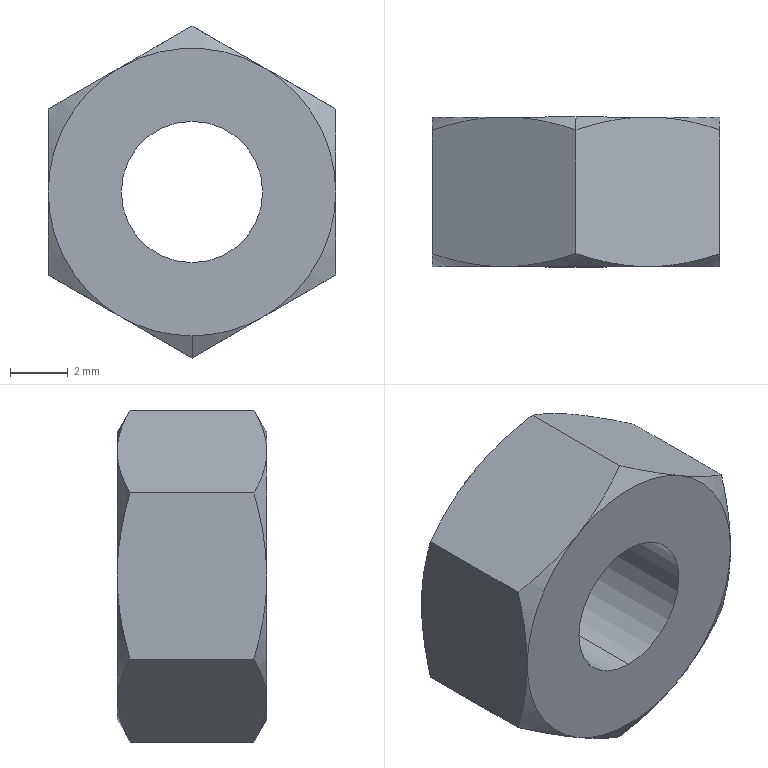Part | STEP file | 1 solid | 24 faces | box 10 x 5.2 x 11.547 mm | volume 349.391 mm3 | cone 14 | plane 8 | cylinder 2 | commonest cylinder face diameters 4.918 x2
STEP:
#1=CARTESIAN_POINT('',(2.5,0.,-4.33));
#2=VERTEX_POINT('',#1);
#3=CARTESIAN_POINT('',(0.,0.,-5.));
#4=VERTEX_POINT('',#3);
#5=CARTESIAN_POINT('',(0.,0.,0.));
#6=DIRECTION('',(0.,1.,0.));
#7=DIRECTION('',(0.,0.,1.));
#8=AXIS2_PLACEMENT_3D('',#5,#6,#7);
#9=CIRCLE('',#8,5.);
#10=EDGE_CURVE('',#2,#4,#9,.T.);
#11=ORIENTED_EDGE('',*,*,#10,.T.);
#12=CARTESIAN_POINT('',(0.,0.4466,-5.774));
#13=VERTEX_POINT('',#12);
#14=CARTESIAN_POINT('',(0.,0.,-5.));
#15=DIRECTION('',(0.,0.5,-0.866));
#16=VECTOR('',#15,1000.);
#17=LINE('',#14,#16);
#18=EDGE_CURVE('',#4,#13,#17,.T.);
#19=ORIENTED_EDGE('',*,*,#18,.T.);
#20=CARTESIAN_POINT('',(0.,0.4466,-5.774));
#21=CARTESIAN_POINT('',(0.8179,0.1739,-5.301));
#22=CARTESIAN_POINT('',(1.648,0.,-4.822));
#23=CARTESIAN_POINT('',(2.5,0.,-4.33));
#24=B_SPLINE_CURVE_WITH_KNOTS('',3,(#20,#21,#22,#23),.UNSPECIFIED.,.F.,.F.,(4,4),(0.000000238,0.002921),.UNSPECIFIED.);
#25=EDGE_CURVE('',#13,#2,#24,.T.);
#26=ORIENTED_EDGE('',*,*,#25,.T.);
#27=EDGE_LOOP('',(#11,#19,#26));
#28=FACE_OUTER_BOUND('',#27,.T.);
#29=CARTESIAN_POINT('',(0.,0.,0.));
#30=DIRECTION('',(0.,1.,0.));
#31=DIRECTION('',(0.,0.,-1.));
#32=AXIS2_PLACEMENT_3D('',#29,#30,#31);
#33=CONICAL_SURFACE('',#32,5.,1.047);
#34=ADVANCED_FACE('',(#28),#33,.T.);
#35=CARTESIAN_POINT('',(0.,5.2,5.));
#36=VERTEX_POINT('',#35);
#37=CARTESIAN_POINT('',(2.5,5.2,4.33));
#38=VERTEX_POINT('',#37);
#39=CARTESIAN_POINT('',(0.,5.2,0.));
#40=DIRECTION('',(0.,1.,0.));
#41=DIRECTION('',(0.,0.,1.));
#42=AXIS2_PLACEMENT_3D('',#39,#40,#41);
#43=CIRCLE('',#42,5.);
#44=EDGE_CURVE('',#36,#38,#43,.T.);
#45=ORIENTED_EDGE('',*,*,#44,.F.);
#46=CARTESIAN_POINT('',(0.,4.753,5.774));
#47=VERTEX_POINT('',#46);
#48=CARTESIAN_POINT('',(0.,5.2,5.));
#49=DIRECTION('',(0.,-0.5,0.866));
#50=VECTOR('',#49,1000.);
#51=LINE('',#48,#50);
#52=EDGE_CURVE('',#36,#47,#51,.T.);
#53=ORIENTED_EDGE('',*,*,#52,.T.);
#54=CARTESIAN_POINT('',(0.,4.753,5.774));
#55=CARTESIAN_POINT('',(0.8179,5.026,5.301));
#56=CARTESIAN_POINT('',(1.648,5.2,4.822));
#57=CARTESIAN_POINT('',(2.5,5.2,4.33));
#58=B_SPLINE_CURVE_WITH_KNOTS('',3,(#54,#55,#56,#57),.UNSPECIFIED.,.F.,.F.,(4,4),(0.000000238,0.002921),.UNSPECIFIED.);
#59=EDGE_CURVE('',#47,#38,#58,.T.);
#60=ORIENTED_EDGE('',*,*,#59,.T.);
#61=EDGE_LOOP('',(#45,#53,#60));
#62=FACE_OUTER_BOUND('',#61,.T.);
#63=CARTESIAN_POINT('',(0.,5.2,0.));
#64=DIRECTION('',(0.,-1.,0.));
#65=DIRECTION('',(0.,0.,1.));
#66=AXIS2_PLACEMENT_3D('',#63,#64,#65);
#67=CONICAL_SURFACE('',#66,5.,1.047);
#68=ADVANCED_FACE('',(#62),#67,.T.);
#69=CARTESIAN_POINT('',(0.,5.2,-2.459));
#70=VERTEX_POINT('',#69);
#71=CARTESIAN_POINT('',(0.,5.2,2.459));
#72=VERTEX_POINT('',#71);
#73=CARTESIAN_POINT('',(0.,5.2,0.));
#74=DIRECTION('',(0.,1.,0.));
#75=DIRECTION('',(0.,0.,1.));
#76=AXIS2_PLACEMENT_3D('',#73,#74,#75);
#77=CIRCLE('',#76,2.459);
#78=EDGE_CURVE('',#70,#72,#77,.T.);
#79=ORIENTED_EDGE('',*,*,#78,.T.);
#80=CARTESIAN_POINT('',(0.,0.,2.459));
#81=VERTEX_POINT('',#80);
#82=CARTESIAN_POINT('',(0.,5.2,2.459));
#83=DIRECTION('',(0.,-1.,0.));
#84=VECTOR('',#83,1000.);
#85=LINE('',#82,#84);
#86=EDGE_CURVE('',#72,#81,#85,.T.);
#87=ORIENTED_EDGE('',*,*,#86,.T.);
#88=CARTESIAN_POINT('',(0.,0.,-2.459));
#89=VERTEX_POINT('',#88);
#90=CARTESIAN_POINT('',(0.,0.,0.));
#91=DIRECTION('',(0.,1.,0.));
#92=DIRECTION('',(0.,0.,1.));
#93=AXIS2_PLACEMENT_3D('',#90,#91,#92);
#94=CIRCLE('',#93,2.459);
#95=EDGE_CURVE('',#89,#81,#94,.T.);
#96=ORIENTED_EDGE('',*,*,#95,.F.);
#97=CARTESIAN_POINT('',(0.,5.2,-2.459));
#98=DIRECTION('',(0.,-1.,0.));
#99=VECTOR('',#98,1000.);
#100=LINE('',#97,#99);
#101=EDGE_CURVE('',#70,#89,#100,.T.);
#102=ORIENTED_EDGE('',*,*,#101,.F.);
#103=EDGE_LOOP('',(#79,#87,#96,#102));
#104=FACE_OUTER_BOUND('',#103,.T.);
#105=CARTESIAN_POINT('',(0.,5.2,0.));
#106=DIRECTION('',(0.,-1.,0.));
#107=DIRECTION('',(0.,0.,-1.));
#108=AXIS2_PLACEMENT_3D('',#105,#106,#107);
#109=CYLINDRICAL_SURFACE('',#108,2.459);
#110=ADVANCED_FACE('',(#104),#109,.F.);
#111=CARTESIAN_POINT('',(-5.,0.4466,-2.887));
#112=VERTEX_POINT('',#111);
#113=CARTESIAN_POINT('',(-2.5,0.,-4.33));
#114=VERTEX_POINT('',#113);
#115=CARTESIAN_POINT('',(-5.,0.4466,-2.887));
#116=CARTESIAN_POINT('',(-4.182,0.1739,-3.359));
#117=CARTESIAN_POINT('',(-3.352,0.,-3.838));
#118=CARTESIAN_POINT('',(-2.5,0.,-4.33));
#119=B_SPLINE_CURVE_WITH_KNOTS('',3,(#115,#116,#117,#118),.UNSPECIFIED.,.F.,.F.,(4,4),(0.000000238,0.002921),.UNSPECIFIED.);
#120=EDGE_CURVE('',#112,#114,#119,.T.);
#121=ORIENTED_EDGE('',*,*,#120,.F.);
#122=CARTESIAN_POINT('',(-5.,4.753,-2.887));
#123=VERTEX_POINT('',#122);
#124=CARTESIAN_POINT('',(-5.,5.2,-2.887));
#125=DIRECTION('',(0.,-1.,0.));
#126=VECTOR('',#125,1000.);
#127=LINE('',#124,#126);
#128=EDGE_CURVE('',#123,#112,#127,.T.);
#129=ORIENTED_EDGE('',*,*,#128,.F.);
#130=CARTESIAN_POINT('',(-2.5,5.2,-4.33));
#131=VERTEX_POINT('',#130);
#132=CARTESIAN_POINT('',(-2.5,5.2,-4.33));
#133=CARTESIAN_POINT('',(-2.712,5.2,-4.208));
#134=CARTESIAN_POINT('',(-2.925,5.189,-4.085));
#135=CARTESIAN_POINT('',(-3.347,5.149,-3.841));
#136=CARTESIAN_POINT('',(-3.556,5.118,-3.72));
#137=CARTESIAN_POINT('',(-4.181,5.002,-3.36));
#138=CARTESIAN_POINT('',(-4.592,4.889,-3.122));
#139=CARTESIAN_POINT('',(-5.,4.753,-2.887));
#140=B_SPLINE_CURVE_WITH_KNOTS('',3,(#132,#133,#134,#135,#136,#137,#138,#139),.UNSPECIFIED.,.F.,.F.,(4,2,2,4),(0.002921,0.003649,0.004376,0.005831),.UNSPECIFIED.);
#141=EDGE_CURVE('',#131,#123,#140,.T.);
#142=ORIENTED_EDGE('',*,*,#141,.F.);
#143=CARTESIAN_POINT('',(0.,4.753,-5.774));
#144=VERTEX_POINT('',#143);
#145=CARTESIAN_POINT('',(0.,4.753,-5.774));
#146=CARTESIAN_POINT('',(-0.8179,5.026,-5.301));
#147=CARTESIAN_POINT('',(-1.648,5.2,-4.822));
#148=CARTESIAN_POINT('',(-2.5,5.2,-4.33));
#149=B_SPLINE_CURVE_WITH_KNOTS('',3,(#145,#146,#147,#148),.UNSPECIFIED.,.F.,.F.,(4,4),(0.000000238,0.002921),.UNSPECIFIED.);
#150=EDGE_CURVE('',#144,#131,#149,.T.);
#151=ORIENTED_EDGE('',*,*,#150,.F.);
#152=CARTESIAN_POINT('',(0.,5.2,-5.774));
#153=DIRECTION('',(0.,-1.,0.));
#154=VECTOR('',#153,1000.);
#155=LINE('',#152,#154);
#156=EDGE_CURVE('',#144,#13,#155,.T.);
#157=ORIENTED_EDGE('',*,*,#156,.T.);
#158=CARTESIAN_POINT('',(-2.5,0.,-4.33));
#159=CARTESIAN_POINT('',(-2.288,0.,-4.453));
#160=CARTESIAN_POINT('',(-2.075,0.01056,-4.576));
#161=CARTESIAN_POINT('',(-1.653,0.0514,-4.819));
#162=CARTESIAN_POINT('',(-1.444,0.08166,-4.94));
#163=CARTESIAN_POINT('',(-0.8193,0.1983,-5.3));
#164=CARTESIAN_POINT('',(-0.4079,0.3106,-5.538));
#165=CARTESIAN_POINT('',(0.,0.4466,-5.774));
#166=B_SPLINE_CURVE_WITH_KNOTS('',3,(#158,#159,#160,#161,#162,#163,#164,#165),.UNSPECIFIED.,.F.,.F.,(4,2,2,4),(0.002921,0.003649,0.004376,0.005831),.UNSPECIFIED.);
#167=EDGE_CURVE('',#114,#13,#166,.T.);
#168=ORIENTED_EDGE('',*,*,#167,.F.);
#169=EDGE_LOOP('',(#121,#129,#142,#151,#157,#168));
#170=FACE_OUTER_BOUND('',#169,.T.);
#171=CARTESIAN_POINT('',(0.,5.2,-5.774));
#172=DIRECTION('',(0.5,0.,0.866));
#173=DIRECTION('',(0.866,0.,-0.5));
#174=AXIS2_PLACEMENT_3D('',#171,#172,#173);
#175=PLANE('',#174);
#176=ADVANCED_FACE('',(#170),#175,.F.);
#177=CARTESIAN_POINT('',(-5.,0.4466,2.887));
#178=VERTEX_POINT('',#177);
#179=CARTESIAN_POINT('',(-5.,0.,0.));
#180=VERTEX_POINT('',#179);
#181=CARTESIAN_POINT('',(-5.,0.4466,2.887));
#182=CARTESIAN_POINT('',(-5.,0.3118,2.42));
#183=CARTESIAN_POINT('',(-5.,0.1996,1.947));
#184=CARTESIAN_POINT('',(-5.,0.04317,0.9834));
#185=CARTESIAN_POINT('',(-5.,0.,0.4885));
#186=CARTESIAN_POINT('',(-5.,0.,0.));
#187=B_SPLINE_CURVE_WITH_KNOTS('',3,(#181,#182,#183,#184,#185,#186),.UNSPECIFIED.,.F.,.F.,(4,2,4),(0.01606,0.01752,0.01898),.UNSPECIFIED.);
#188=EDGE_CURVE('',#178,#180,#187,.T.);
#189=ORIENTED_EDGE('',*,*,#188,.F.);
#190=CARTESIAN_POINT('',(-5.,4.753,2.887));
#191=VERTEX_POINT('',#190);
#192=CARTESIAN_POINT('',(-5.,5.2,2.887));
#193=DIRECTION('',(0.,-1.,0.));
#194=VECTOR('',#193,1000.);
#195=LINE('',#192,#194);
#196=EDGE_CURVE('',#191,#178,#195,.T.);
#197=ORIENTED_EDGE('',*,*,#196,.F.);
#198=CARTESIAN_POINT('',(-5.,5.2,0.));
#199=VERTEX_POINT('',#198);
#200=CARTESIAN_POINT('',(-5.,5.2,0.));
#201=CARTESIAN_POINT('',(-5.,5.2,0.4885));
#202=CARTESIAN_POINT('',(-5.,5.157,0.9834));
#203=CARTESIAN_POINT('',(-5.,5.,1.947));
#204=CARTESIAN_POINT('',(-5.,4.888,2.42));
#205=CARTESIAN_POINT('',(-5.,4.753,2.887));
#206=B_SPLINE_CURVE_WITH_KNOTS('',3,(#200,#201,#202,#203,#204,#205),.UNSPECIFIED.,.F.,.F.,(4,2,4),(0.008187,0.009649,0.01111),.UNSPECIFIED.);
#207=EDGE_CURVE('',#199,#191,#206,.T.);
#208=ORIENTED_EDGE('',*,*,#207,.F.);
#209=CARTESIAN_POINT('',(-5.,4.753,-2.887));
#210=CARTESIAN_POINT('',(-5.,4.889,-2.417));
#211=CARTESIAN_POINT('',(-5.,5.003,-1.936));
#212=CARTESIAN_POINT('',(-5.,5.158,-0.9728));
#213=CARTESIAN_POINT('',(-5.,5.2,-0.4881));
#214=CARTESIAN_POINT('',(-5.,5.2,0.));
#215=B_SPLINE_CURVE_WITH_KNOTS('',3,(#209,#210,#211,#212,#213,#214),.UNSPECIFIED.,.F.,.F.,(4,2,4),(0.005265,0.006726,0.008187),.UNSPECIFIED.);
#216=EDGE_CURVE('',#123,#199,#215,.T.);
#217=ORIENTED_EDGE('',*,*,#216,.F.);
#218=ORIENTED_EDGE('',*,*,#128,.T.);
#219=CARTESIAN_POINT('',(-5.,0.,0.));
#220=CARTESIAN_POINT('',(-5.,0.,-0.4881));
#221=CARTESIAN_POINT('',(-5.,0.04198,-0.9728));
#222=CARTESIAN_POINT('',(-5.,0.1973,-1.936));
#223=CARTESIAN_POINT('',(-5.,0.311,-2.417));
#224=CARTESIAN_POINT('',(-5.,0.4466,-2.887));
#225=B_SPLINE_CURVE_WITH_KNOTS('',3,(#219,#220,#221,#222,#223,#224),.UNSPECIFIED.,.F.,.F.,(4,2,4),(0.01898,0.02045,0.02191),.UNSPECIFIED.);
#226=EDGE_CURVE('',#180,#112,#225,.T.);
#227=ORIENTED_EDGE('',*,*,#226,.F.);
#228=EDGE_LOOP('',(#189,#197,#208,#217,#218,#227));
#229=FACE_OUTER_BOUND('',#228,.T.);
#230=CARTESIAN_POINT('',(-5.,5.2,-2.887));
#231=DIRECTION('',(1.,0.,0.));
#232=DIRECTION('',(0.,0.,-1.));
#233=AXIS2_PLACEMENT_3D('',#230,#231,#232);
#234=PLANE('',#233);
#235=ADVANCED_FACE('',(#229),#234,.F.);
#236=CARTESIAN_POINT('',(0.,0.4466,5.774));
#237=VERTEX_POINT('',#236);
#238=CARTESIAN_POINT('',(-2.5,0.,4.33));
#239=VERTEX_POINT('',#238);
#240=CARTESIAN_POINT('',(0.,0.4466,5.774));
#241=CARTESIAN_POINT('',(-0.8179,0.1739,5.301));
#242=CARTESIAN_POINT('',(-1.648,0.,4.822));
#243=CARTESIAN_POINT('',(-2.5,0.,4.33));
#244=B_SPLINE_CURVE_WITH_KNOTS('',3,(#240,#241,#242,#243),.UNSPECIFIED.,.F.,.F.,(4,4),(0.000000238,0.002921),.UNSPECIFIED.);
#245=EDGE_CURVE('',#237,#239,#244,.T.);
#246=ORIENTED_EDGE('',*,*,#245,.F.);
#247=CARTESIAN_POINT('',(0.,5.2,5.774));
#248=DIRECTION('',(0.,-1.,0.));
#249=VECTOR('',#248,1000.);
#250=LINE('',#247,#249);
#251=EDGE_CURVE('',#47,#237,#250,.T.);
#252=ORIENTED_EDGE('',*,*,#251,.F.);
#253=CARTESIAN_POINT('',(-2.5,5.2,4.33));
#254=VERTEX_POINT('',#253);
#255=CARTESIAN_POINT('',(-2.5,5.2,4.33));
#256=CARTESIAN_POINT('',(-2.288,5.2,4.453));
#257=CARTESIAN_POINT('',(-2.075,5.189,4.576));
#258=CARTESIAN_POINT('',(-1.653,5.149,4.819));
#259=CARTESIAN_POINT('',(-1.444,5.118,4.94));
#260=CARTESIAN_POINT('',(-0.8193,5.002,5.3));
#261=CARTESIAN_POINT('',(-0.4079,4.889,5.538));
#262=CARTESIAN_POINT('',(0.,4.753,5.774));
#263=B_SPLINE_CURVE_WITH_KNOTS('',3,(#255,#256,#257,#258,#259,#260,#261,#262),.UNSPECIFIED.,.F.,.F.,(4,2,2,4),(0.002921,0.003649,0.004376,0.005831),.UNSPECIFIED.);
#264=EDGE_CURVE('',#254,#47,#263,.T.);
#265=ORIENTED_EDGE('',*,*,#264,.F.);
#266=CARTESIAN_POINT('',(-5.,4.753,2.887));
#267=CARTESIAN_POINT('',(-4.182,5.026,3.359));
#268=CARTESIAN_POINT('',(-3.352,5.2,3.838));
#269=CARTESIAN_POINT('',(-2.5,5.2,4.33));
#270=B_SPLINE_CURVE_WITH_KNOTS('',3,(#266,#267,#268,#269),.UNSPECIFIED.,.F.,.F.,(4,4),(0.000000238,0.002921),.UNSPECIFIED.);
#271=EDGE_CURVE('',#191,#254,#270,.T.);
#272=ORIENTED_EDGE('',*,*,#271,.F.);
#273=ORIENTED_EDGE('',*,*,#196,.T.);
#274=CARTESIAN_POINT('',(-2.5,0.,4.33));
#275=CARTESIAN_POINT('',(-2.712,0.,4.208));
#276=CARTESIAN_POINT('',(-2.925,0.01056,4.085));
#277=CARTESIAN_POINT('',(-3.347,0.0514,3.841));
#278=CARTESIAN_POINT('',(-3.556,0.08166,3.72));
#279=CARTESIAN_POINT('',(-4.181,0.1983,3.36));
#280=CARTESIAN_POINT('',(-4.592,0.3106,3.122));
#281=CARTESIAN_POINT('',(-5.,0.4466,2.887));
#282=B_SPLINE_CURVE_WITH_KNOTS('',3,(#274,#275,#276,#277,#278,#279,#280,#281),.UNSPECIFIED.,.F.,.F.,(4,2,2,4),(0.002921,0.003649,0.004376,0.005831),.UNSPECIFIED.);
#283=EDGE_CURVE('',#239,#178,#282,.T.);
#284=ORIENTED_EDGE('',*,*,#283,.F.);
#285=EDGE_LOOP('',(#246,#252,#265,#272,#273,#284));
#286=FACE_OUTER_BOUND('',#285,.T.);
#287=CARTESIAN_POINT('',(-5.,5.2,2.887));
#288=DIRECTION('',(0.5,0.,-0.866));
#289=DIRECTION('',(-0.866,0.,-0.5));
#290=AXIS2_PLACEMENT_3D('',#287,#288,#289);
#291=PLANE('',#290);
#292=ADVANCED_FACE('',(#286),#291,.F.);
#293=CARTESIAN_POINT('',(5.,0.4466,2.887));
#294=VERTEX_POINT('',#293);
#295=CARTESIAN_POINT('',(2.5,0.,4.33));
#296=VERTEX_POINT('',#295);
#297=CARTESIAN_POINT('',(5.,0.4466,2.887));
#298=CARTESIAN_POINT('',(4.182,0.1739,3.359));
#299=CARTESIAN_POINT('',(3.352,0.,3.838));
#300=CARTESIAN_POINT('',(2.5,0.,4.33));
#301=B_SPLINE_CURVE_WITH_KNOTS('',3,(#297,#298,#299,#300),.UNSPECIFIED.,.F.,.F.,(4,4),(0.000000238,0.002921),.UNSPECIFIED.);
#302=EDGE_CURVE('',#294,#296,#301,.T.);
#303=ORIENTED_EDGE('',*,*,#302,.F.);
#304=CARTESIAN_POINT('',(5.,4.753,2.887));
#305=VERTEX_POINT('',#304);
#306=CARTESIAN_POINT('',(5.,5.2,2.887));
#307=DIRECTION('',(0.,-1.,0.));
#308=VECTOR('',#307,1000.);
#309=LINE('',#306,#308);
#310=EDGE_CURVE('',#305,#294,#309,.T.);
#311=ORIENTED_EDGE('',*,*,#310,.F.);
#312=CARTESIAN_POINT('',(2.5,5.2,4.33));
#313=CARTESIAN_POINT('',(2.712,5.2,4.208));
#314=CARTESIAN_POINT('',(2.925,5.189,4.085));
#315=CARTESIAN_POINT('',(3.347,5.149,3.841));
#316=CARTESIAN_POINT('',(3.556,5.118,3.72));
#317=CARTESIAN_POINT('',(4.181,5.002,3.36));
#318=CARTESIAN_POINT('',(4.592,4.889,3.122));
#319=CARTESIAN_POINT('',(5.,4.753,2.887));
#320=B_SPLINE_CURVE_WITH_KNOTS('',3,(#312,#313,#314,#315,#316,#317,#318,#319),.UNSPECIFIED.,.F.,.F.,(4,2,2,4),(0.002921,0.003649,0.004376,0.005831),.UNSPECIFIED.);
#321=EDGE_CURVE('',#38,#305,#320,.T.);
#322=ORIENTED_EDGE('',*,*,#321,.F.);
#323=ORIENTED_EDGE('',*,*,#59,.F.);
#324=ORIENTED_EDGE('',*,*,#251,.T.);
#325=CARTESIAN_POINT('',(2.5,0.,4.33));
#326=CARTESIAN_POINT('',(2.288,0.,4.453));
#327=CARTESIAN_POINT('',(2.075,0.01056,4.576));
#328=CARTESIAN_POINT('',(1.653,0.0514,4.819));
#329=CARTESIAN_POINT('',(1.444,0.08166,4.94));
#330=CARTESIAN_POINT('',(0.8193,0.1983,5.3));
#331=CARTESIAN_POINT('',(0.4079,0.3106,5.538));
#332=CARTESIAN_POINT('',(0.,0.4466,5.774));
#333=B_SPLINE_CURVE_WITH_KNOTS('',3,(#325,#326,#327,#328,#329,#330,#331,#332),.UNSPECIFIED.,.F.,.F.,(4,2,2,4),(0.002921,0.003649,0.004376,0.005831),.UNSPECIFIED.);
#334=EDGE_CURVE('',#296,#237,#333,.T.);
#335=ORIENTED_EDGE('',*,*,#334,.F.);
#336=EDGE_LOOP('',(#303,#311,#322,#323,#324,#335));
#337=FACE_OUTER_BOUND('',#336,.T.);
#338=CARTESIAN_POINT('',(0.,5.2,5.774));
#339=DIRECTION('',(-0.5,0.,-0.866));
#340=DIRECTION('',(-0.866,0.,0.5));
#341=AXIS2_PLACEMENT_3D('',#338,#339,#340);
#342=PLANE('',#341);
#343=ADVANCED_FACE('',(#337),#342,.F.);
#344=CARTESIAN_POINT('',(5.,0.4466,-2.887));
#345=VERTEX_POINT('',#344);
#346=CARTESIAN_POINT('',(5.,0.,0.));
#347=VERTEX_POINT('',#346);
#348=CARTESIAN_POINT('',(5.,0.4466,-2.887));
#349=CARTESIAN_POINT('',(5.,0.311,-2.417));
#350=CARTESIAN_POINT('',(5.,0.1973,-1.936));
#351=CARTESIAN_POINT('',(5.,0.04198,-0.9728));
#352=CARTESIAN_POINT('',(5.,0.,-0.4881));
#353=CARTESIAN_POINT('',(5.,0.,0.));
#354=B_SPLINE_CURVE_WITH_KNOTS('',3,(#348,#349,#350,#351,#352,#353),.UNSPECIFIED.,.F.,.F.,(4,2,4),(0.005265,0.006726,0.008187),.UNSPECIFIED.);
#355=EDGE_CURVE('',#345,#347,#354,.T.);
#356=ORIENTED_EDGE('',*,*,#355,.F.);
#357=CARTESIAN_POINT('',(5.,4.753,-2.887));
#358=VERTEX_POINT('',#357);
#359=CARTESIAN_POINT('',(5.,5.2,-2.887));
#360=DIRECTION('',(0.,-1.,0.));
#361=VECTOR('',#360,1000.);
#362=LINE('',#359,#361);
#363=EDGE_CURVE('',#358,#345,#362,.T.);
#364=ORIENTED_EDGE('',*,*,#363,.F.);
#365=CARTESIAN_POINT('',(5.,5.2,0.));
#366=VERTEX_POINT('',#365);
#367=CARTESIAN_POINT('',(5.,5.2,0.));
#368=CARTESIAN_POINT('',(5.,5.2,-0.4881));
#369=CARTESIAN_POINT('',(5.,5.158,-0.9728));
#370=CARTESIAN_POINT('',(5.,5.003,-1.936));
#371=CARTESIAN_POINT('',(5.,4.889,-2.417));
#372=CARTESIAN_POINT('',(5.,4.753,-2.887));
#373=B_SPLINE_CURVE_WITH_KNOTS('',3,(#367,#368,#369,#370,#371,#372),.UNSPECIFIED.,.F.,.F.,(4,2,4),(0.01898,0.02045,0.02191),.UNSPECIFIED.);
#374=EDGE_CURVE('',#366,#358,#373,.T.);
#375=ORIENTED_EDGE('',*,*,#374,.F.);
#376=CARTESIAN_POINT('',(5.,4.753,2.887));
#377=CARTESIAN_POINT('',(5.,4.888,2.42));
#378=CARTESIAN_POINT('',(5.,5.,1.947));
#379=CARTESIAN_POINT('',(5.,5.157,0.9834));
#380=CARTESIAN_POINT('',(5.,5.2,0.4885));
#381=CARTESIAN_POINT('',(5.,5.2,0.));
#382=B_SPLINE_CURVE_WITH_KNOTS('',3,(#376,#377,#378,#379,#380,#381),.UNSPECIFIED.,.F.,.F.,(4,2,4),(0.01606,0.01752,0.01898),.UNSPECIFIED.);
#383=EDGE_CURVE('',#305,#366,#382,.T.);
#384=ORIENTED_EDGE('',*,*,#383,.F.);
#385=ORIENTED_EDGE('',*,*,#310,.T.);
#386=CARTESIAN_POINT('',(5.,0.,0.));
#387=CARTESIAN_POINT('',(5.,0.,0.4885));
#388=CARTESIAN_POINT('',(5.,0.04317,0.9834));
#389=CARTESIAN_POINT('',(5.,0.1996,1.947));
#390=CARTESIAN_POINT('',(5.,0.3118,2.42));
#391=CARTESIAN_POINT('',(5.,0.4466,2.887));
#392=B_SPLINE_CURVE_WITH_KNOTS('',3,(#386,#387,#388,#389,#390,#391),.UNSPECIFIED.,.F.,.F.,(4,2,4),(0.008187,0.009649,0.01111),.UNSPECIFIED.);
#393=EDGE_CURVE('',#347,#294,#392,.T.);
#394=ORIENTED_EDGE('',*,*,#393,.F.);
#395=EDGE_LOOP('',(#356,#364,#375,#384,#385,#394));
#396=FACE_OUTER_BOUND('',#395,.T.);
#397=CARTESIAN_POINT('',(5.,5.2,2.887));
#398=DIRECTION('',(-1.,0.,0.));
#399=DIRECTION('',(0.,0.,1.));
#400=AXIS2_PLACEMENT_3D('',#397,#398,#399);
#401=PLANE('',#400);
#402=ADVANCED_FACE('',(#396),#401,.F.);
#403=ORIENTED_EDGE('',*,*,#25,.F.);
#404=ORIENTED_EDGE('',*,*,#156,.F.);
#405=CARTESIAN_POINT('',(2.5,5.2,-4.33));
#406=VERTEX_POINT('',#405);
#407=CARTESIAN_POINT('',(2.5,5.2,-4.33));
#408=CARTESIAN_POINT('',(2.288,5.2,-4.453));
#409=CARTESIAN_POINT('',(2.075,5.189,-4.576));
#410=CARTESIAN_POINT('',(1.653,5.149,-4.819));
#411=CARTESIAN_POINT('',(1.444,5.118,-4.94));
#412=CARTESIAN_POINT('',(0.8193,5.002,-5.3));
#413=CARTESIAN_POINT('',(0.4079,4.889,-5.538));
#414=CARTESIAN_POINT('',(0.,4.753,-5.774));
#415=B_SPLINE_CURVE_WITH_KNOTS('',3,(#407,#408,#409,#410,#411,#412,#413,#414),.UNSPECIFIED.,.F.,.F.,(4,2,2,4),(0.002921,0.003649,0.004376,0.005831),.UNSPECIFIED.);
#416=EDGE_CURVE('',#406,#144,#415,.T.);
#417=ORIENTED_EDGE('',*,*,#416,.F.);
#418=CARTESIAN_POINT('',(5.,4.753,-2.887));
#419=CARTESIAN_POINT('',(4.182,5.026,-3.359));
#420=CARTESIAN_POINT('',(3.352,5.2,-3.838));
#421=CARTESIAN_POINT('',(2.5,5.2,-4.33));
#422=B_SPLINE_CURVE_WITH_KNOTS('',3,(#418,#419,#420,#421),.UNSPECIFIED.,.F.,.F.,(4,4),(0.000000238,0.002921),.UNSPECIFIED.);
#423=EDGE_CURVE('',#358,#406,#422,.T.);
#424=ORIENTED_EDGE('',*,*,#423,.F.);
#425=ORIENTED_EDGE('',*,*,#363,.T.);
#426=CARTESIAN_POINT('',(2.5,0.,-4.33));
#427=CARTESIAN_POINT('',(2.712,0.,-4.208));
#428=CARTESIAN_POINT('',(2.925,0.01056,-4.085));
#429=CARTESIAN_POINT('',(3.347,0.0514,-3.841));
#430=CARTESIAN_POINT('',(3.556,0.08166,-3.72));
#431=CARTESIAN_POINT('',(4.181,0.1983,-3.36));
#432=CARTESIAN_POINT('',(4.592,0.3106,-3.122));
#433=CARTESIAN_POINT('',(5.,0.4466,-2.887));
#434=B_SPLINE_CURVE_WITH_KNOTS('',3,(#426,#427,#428,#429,#430,#431,#432,#433),.UNSPECIFIED.,.F.,.F.,(4,2,2,4),(0.002921,0.003649,0.004376,0.005831),.UNSPECIFIED.);
#435=EDGE_CURVE('',#2,#345,#434,.T.);
#436=ORIENTED_EDGE('',*,*,#435,.F.);
#437=EDGE_LOOP('',(#403,#404,#417,#424,#425,#436));
#438=FACE_OUTER_BOUND('',#437,.T.);
#439=CARTESIAN_POINT('',(5.,5.2,-2.887));
#440=DIRECTION('',(-0.5,0.,0.866));
#441=DIRECTION('',(0.866,0.,0.5));
#442=AXIS2_PLACEMENT_3D('',#439,#440,#441);
#443=PLANE('',#442);
#444=ADVANCED_FACE('',(#438),#443,.F.);
#445=ORIENTED_EDGE('',*,*,#95,.T.);
#446=CARTESIAN_POINT('',(0.,0.,0.));
#447=DIRECTION('',(0.,1.,0.));
#448=DIRECTION('',(0.,0.,1.));
#449=AXIS2_PLACEMENT_3D('',#446,#447,#448);
#450=CIRCLE('',#449,2.459);
#451=EDGE_CURVE('',#81,#89,#450,.T.);
#452=ORIENTED_EDGE('',*,*,#451,.T.);
#453=EDGE_LOOP('',(#445,#452));
#454=FACE_BOUND('',#453,.T.);
#455=CARTESIAN_POINT('',(0.,0.,0.));
#456=DIRECTION('',(0.,1.,0.));
#457=DIRECTION('',(0.,0.,1.));
#458=AXIS2_PLACEMENT_3D('',#455,#456,#457);
#459=CIRCLE('',#458,5.);
#460=EDGE_CURVE('',#296,#347,#459,.T.);
#461=ORIENTED_EDGE('',*,*,#460,.F.);
#462=CARTESIAN_POINT('',(0.,0.,0.));
#463=DIRECTION('',(0.,1.,0.));
#464=DIRECTION('',(0.,0.,1.));
#465=AXIS2_PLACEMENT_3D('',#462,#463,#464);
#466=CIRCLE('',#465,5.);
#467=EDGE_CURVE('',#239,#296,#466,.T.);
#468=ORIENTED_EDGE('',*,*,#467,.F.);
#469=CARTESIAN_POINT('',(0.,0.,0.));
#470=DIRECTION('',(0.,1.,0.));
#471=DIRECTION('',(0.,0.,1.));
#472=AXIS2_PLACEMENT_3D('',#469,#470,#471);
#473=CIRCLE('',#472,5.);
#474=EDGE_CURVE('',#180,#239,#473,.T.);
#475=ORIENTED_EDGE('',*,*,#474,.F.);
#476=CARTESIAN_POINT('',(0.,0.,0.));
#477=DIRECTION('',(0.,1.,0.));
#478=DIRECTION('',(0.,0.,1.));
#479=AXIS2_PLACEMENT_3D('',#476,#477,#478);
#480=CIRCLE('',#479,5.);
#481=EDGE_CURVE('',#114,#180,#480,.T.);
#482=ORIENTED_EDGE('',*,*,#481,.F.);
#483=CARTESIAN_POINT('',(0.,0.,0.));
#484=DIRECTION('',(0.,1.,0.));
#485=DIRECTION('',(0.,0.,1.));
#486=AXIS2_PLACEMENT_3D('',#483,#484,#485);
#487=CIRCLE('',#486,5.);
#488=EDGE_CURVE('',#4,#114,#487,.T.);
#489=ORIENTED_EDGE('',*,*,#488,.F.);
#490=ORIENTED_EDGE('',*,*,#10,.F.);
#491=CARTESIAN_POINT('',(0.,0.,0.));
#492=DIRECTION('',(0.,-1.,0.));
#493=DIRECTION('',(0.,0.,-1.));
#494=AXIS2_PLACEMENT_3D('',#491,#492,#493);
#495=CIRCLE('',#494,5.);
#496=EDGE_CURVE('',#2,#347,#495,.T.);
#497=ORIENTED_EDGE('',*,*,#496,.T.);
#498=EDGE_LOOP('',(#461,#468,#475,#482,#489,#490,#497));
#499=FACE_OUTER_BOUND('',#498,.T.);
#500=CARTESIAN_POINT('',(0.,0.,0.));
#501=DIRECTION('',(0.,1.,0.));
#502=DIRECTION('',(0.,0.,1.));
#503=AXIS2_PLACEMENT_3D('',#500,#501,#502);
#504=PLANE('',#503);
#505=ADVANCED_FACE('',(#454,#499),#504,.F.);
#506=ORIENTED_EDGE('',*,*,#78,.F.);
#507=CARTESIAN_POINT('',(0.,5.2,0.));
#508=DIRECTION('',(0.,1.,0.));
#509=DIRECTION('',(0.,0.,1.));
#510=AXIS2_PLACEMENT_3D('',#507,#508,#509);
#511=CIRCLE('',#510,2.459);
#512=EDGE_CURVE('',#72,#70,#511,.T.);
#513=ORIENTED_EDGE('',*,*,#512,.F.);
#514=EDGE_LOOP('',(#506,#513));
#515=FACE_BOUND('',#514,.T.);
#516=CARTESIAN_POINT('',(0.,5.2,0.));
#517=DIRECTION('',(0.,1.,0.));
#518=DIRECTION('',(0.,0.,1.));
#519=AXIS2_PLACEMENT_3D('',#516,#517,#518);
#520=CIRCLE('',#519,5.);
#521=EDGE_CURVE('',#254,#36,#520,.T.);
#522=ORIENTED_EDGE('',*,*,#521,.T.);
#523=ORIENTED_EDGE('',*,*,#44,.T.);
#524=CARTESIAN_POINT('',(0.,5.2,0.));
#525=DIRECTION('',(0.,1.,0.));
#526=DIRECTION('',(0.,0.,1.));
#527=AXIS2_PLACEMENT_3D('',#524,#525,#526);
#528=CIRCLE('',#527,5.);
#529=EDGE_CURVE('',#38,#366,#528,.T.);
#530=ORIENTED_EDGE('',*,*,#529,.T.);
#531=CARTESIAN_POINT('',(0.,5.2,0.));
#532=DIRECTION('',(0.,1.,0.));
#533=DIRECTION('',(0.,0.,1.));
#534=AXIS2_PLACEMENT_3D('',#531,#532,#533);
#535=CIRCLE('',#534,5.);
#536=EDGE_CURVE('',#366,#406,#535,.T.);
#537=ORIENTED_EDGE('',*,*,#536,.T.);
#538=CARTESIAN_POINT('',(0.,5.2,0.));
#539=DIRECTION('',(0.,1.,0.));
#540=DIRECTION('',(0.,0.,1.));
#541=AXIS2_PLACEMENT_3D('',#538,#539,#540);
#542=CIRCLE('',#541,5.);
#543=EDGE_CURVE('',#406,#131,#542,.T.);
#544=ORIENTED_EDGE('',*,*,#543,.T.);
#545=CARTESIAN_POINT('',(0.,5.2,0.));
#546=DIRECTION('',(0.,1.,0.));
#547=DIRECTION('',(0.,0.,1.));
#548=AXIS2_PLACEMENT_3D('',#545,#546,#547);
#549=CIRCLE('',#548,5.);
#550=EDGE_CURVE('',#131,#199,#549,.T.);
#551=ORIENTED_EDGE('',*,*,#550,.T.);
#552=CARTESIAN_POINT('',(0.,5.2,0.));
#553=DIRECTION('',(0.,1.,0.));
#554=DIRECTION('',(0.,0.,1.));
#555=AXIS2_PLACEMENT_3D('',#552,#553,#554);
#556=CIRCLE('',#555,5.);
#557=EDGE_CURVE('',#199,#254,#556,.T.);
#558=ORIENTED_EDGE('',*,*,#557,.T.);
#559=EDGE_LOOP('',(#522,#523,#530,#537,#544,#551,#558));
#560=FACE_OUTER_BOUND('',#559,.T.);
#561=CARTESIAN_POINT('',(0.,5.2,0.));
#562=DIRECTION('',(0.,1.,0.));
#563=DIRECTION('',(0.,0.,1.));
#564=AXIS2_PLACEMENT_3D('',#561,#562,#563);
#565=PLANE('',#564);
#566=ADVANCED_FACE('',(#515,#560),#565,.T.);
#567=ORIENTED_EDGE('',*,*,#86,.F.);
#568=ORIENTED_EDGE('',*,*,#512,.T.);
#569=ORIENTED_EDGE('',*,*,#101,.T.);
#570=ORIENTED_EDGE('',*,*,#451,.F.);
#571=EDGE_LOOP('',(#567,#568,#569,#570));
#572=FACE_OUTER_BOUND('',#571,.T.);
#573=CARTESIAN_POINT('',(0.,5.2,0.));
#574=DIRECTION('',(0.,-1.,0.));
#575=DIRECTION('',(0.,0.,-1.));
#576=AXIS2_PLACEMENT_3D('',#573,#574,#575);
#577=CYLINDRICAL_SURFACE('',#576,2.459);
#578=ADVANCED_FACE('',(#572),#577,.F.);
#579=ORIENTED_EDGE('',*,*,#150,.T.);
#580=ORIENTED_EDGE('',*,*,#543,.F.);
#581=ORIENTED_EDGE('',*,*,#416,.T.);
#582=EDGE_LOOP('',(#579,#580,#581));
#583=FACE_OUTER_BOUND('',#582,.T.);
#584=CARTESIAN_POINT('',(0.,5.2,0.));
#585=DIRECTION('',(0.,-1.,0.));
#586=DIRECTION('',(0.,0.,1.));
#587=AXIS2_PLACEMENT_3D('',#584,#585,#586);
#588=CONICAL_SURFACE('',#587,5.,1.047);
#589=ADVANCED_FACE('',(#583),#588,.T.);
#590=ORIENTED_EDGE('',*,*,#374,.T.);
#591=ORIENTED_EDGE('',*,*,#423,.T.);
#592=ORIENTED_EDGE('',*,*,#536,.F.);
#593=EDGE_LOOP('',(#590,#591,#592));
#594=FACE_OUTER_BOUND('',#593,.T.);
#595=CARTESIAN_POINT('',(0.,5.2,0.));
#596=DIRECTION('',(0.,-1.,0.));
#597=DIRECTION('',(0.,0.,1.));
#598=AXIS2_PLACEMENT_3D('',#595,#596,#597);
#599=CONICAL_SURFACE('',#598,5.,1.047);
#600=ADVANCED_FACE('',(#594),#599,.T.);
#601=ORIENTED_EDGE('',*,*,#321,.T.);
#602=ORIENTED_EDGE('',*,*,#383,.T.);
#603=ORIENTED_EDGE('',*,*,#529,.F.);
#604=EDGE_LOOP('',(#601,#602,#603));
#605=FACE_OUTER_BOUND('',#604,.T.);
#606=CARTESIAN_POINT('',(0.,5.2,0.));
#607=DIRECTION('',(0.,-1.,0.));
#608=DIRECTION('',(0.,0.,1.));
#609=AXIS2_PLACEMENT_3D('',#606,#607,#608);
#610=CONICAL_SURFACE('',#609,5.,1.047);
#611=ADVANCED_FACE('',(#605),#610,.T.);
#612=ORIENTED_EDGE('',*,*,#52,.F.);
#613=ORIENTED_EDGE('',*,*,#521,.F.);
#614=ORIENTED_EDGE('',*,*,#264,.T.);
#615=EDGE_LOOP('',(#612,#613,#614));
#616=FACE_OUTER_BOUND('',#615,.T.);
#617=CARTESIAN_POINT('',(0.,5.2,0.));
#618=DIRECTION('',(0.,-1.,0.));
#619=DIRECTION('',(0.,0.,1.));
#620=AXIS2_PLACEMENT_3D('',#617,#618,#619);
#621=CONICAL_SURFACE('',#620,5.,1.047);
#622=ADVANCED_FACE('',(#616),#621,.T.);
#623=ORIENTED_EDGE('',*,*,#207,.T.);
#624=ORIENTED_EDGE('',*,*,#271,.T.);
#625=ORIENTED_EDGE('',*,*,#557,.F.);
#626=EDGE_LOOP('',(#623,#624,#625));
#627=FACE_OUTER_BOUND('',#626,.T.);
#628=CARTESIAN_POINT('',(0.,5.2,0.));
#629=DIRECTION('',(0.,-1.,0.));
#630=DIRECTION('',(0.,0.,1.));
#631=AXIS2_PLACEMENT_3D('',#628,#629,#630);
#632=CONICAL_SURFACE('',#631,5.,1.047);
#633=ADVANCED_FACE('',(#627),#632,.T.);
#634=ORIENTED_EDGE('',*,*,#141,.T.);
#635=ORIENTED_EDGE('',*,*,#216,.T.);
#636=ORIENTED_EDGE('',*,*,#550,.F.);
#637=EDGE_LOOP('',(#634,#635,#636));
#638=FACE_OUTER_BOUND('',#637,.T.);
#639=CARTESIAN_POINT('',(0.,5.2,0.));
#640=DIRECTION('',(0.,-1.,0.));
#641=DIRECTION('',(0.,0.,1.));
#642=AXIS2_PLACEMENT_3D('',#639,#640,#641);
#643=CONICAL_SURFACE('',#642,5.,1.047);
#644=ADVANCED_FACE('',(#638),#643,.T.);
#645=ORIENTED_EDGE('',*,*,#245,.T.);
#646=ORIENTED_EDGE('',*,*,#467,.T.);
#647=ORIENTED_EDGE('',*,*,#334,.T.);
#648=EDGE_LOOP('',(#645,#646,#647));
#649=FACE_OUTER_BOUND('',#648,.T.);
#650=CARTESIAN_POINT('',(0.,0.,0.));
#651=DIRECTION('',(0.,1.,0.));
#652=DIRECTION('',(0.,0.,-1.));
#653=AXIS2_PLACEMENT_3D('',#650,#651,#652);
#654=CONICAL_SURFACE('',#653,5.,1.047);
#655=ADVANCED_FACE('',(#649),#654,.T.);
#656=ORIENTED_EDGE('',*,*,#283,.T.);
#657=ORIENTED_EDGE('',*,*,#188,.T.);
#658=ORIENTED_EDGE('',*,*,#474,.T.);
#659=EDGE_LOOP('',(#656,#657,#658));
#660=FACE_OUTER_BOUND('',#659,.T.);
#661=CARTESIAN_POINT('',(0.,0.,0.));
#662=DIRECTION('',(0.,1.,0.));
#663=DIRECTION('',(0.,0.,-1.));
#664=AXIS2_PLACEMENT_3D('',#661,#662,#663);
#665=CONICAL_SURFACE('',#664,5.,1.047);
#666=ADVANCED_FACE('',(#660),#665,.T.);
#667=ORIENTED_EDGE('',*,*,#226,.T.);
#668=ORIENTED_EDGE('',*,*,#120,.T.);
#669=ORIENTED_EDGE('',*,*,#481,.T.);
#670=EDGE_LOOP('',(#667,#668,#669));
#671=FACE_OUTER_BOUND('',#670,.T.);
#672=CARTESIAN_POINT('',(0.,0.,0.));
#673=DIRECTION('',(0.,1.,0.));
#674=DIRECTION('',(0.,0.,-1.));
#675=AXIS2_PLACEMENT_3D('',#672,#673,#674);
#676=CONICAL_SURFACE('',#675,5.,1.047);
#677=ADVANCED_FACE('',(#671),#676,.T.);
#678=ORIENTED_EDGE('',*,*,#18,.F.);
#679=ORIENTED_EDGE('',*,*,#488,.T.);
#680=ORIENTED_EDGE('',*,*,#167,.T.);
#681=EDGE_LOOP('',(#678,#679,#680));
#682=FACE_OUTER_BOUND('',#681,.T.);
#683=CARTESIAN_POINT('',(0.,0.,0.));
#684=DIRECTION('',(0.,1.,0.));
#685=DIRECTION('',(0.,0.,-1.));
#686=AXIS2_PLACEMENT_3D('',#683,#684,#685);
#687=CONICAL_SURFACE('',#686,5.,1.047);
#688=ADVANCED_FACE('',(#682),#687,.T.);
#689=ORIENTED_EDGE('',*,*,#355,.T.);
#690=ORIENTED_EDGE('',*,*,#496,.F.);
#691=ORIENTED_EDGE('',*,*,#435,.T.);
#692=EDGE_LOOP('',(#689,#690,#691));
#693=FACE_OUTER_BOUND('',#692,.T.);
#694=CARTESIAN_POINT('',(0.,0.,0.));
#695=DIRECTION('',(0.,1.,0.));
#696=DIRECTION('',(0.,0.,-1.));
#697=AXIS2_PLACEMENT_3D('',#694,#695,#696);
#698=CONICAL_SURFACE('',#697,5.,1.047);
#699=ADVANCED_FACE('',(#693),#698,.T.);
#700=ORIENTED_EDGE('',*,*,#302,.T.);
#701=ORIENTED_EDGE('',*,*,#460,.T.);
#702=ORIENTED_EDGE('',*,*,#393,.T.);
#703=EDGE_LOOP('',(#700,#701,#702));
#704=FACE_OUTER_BOUND('',#703,.T.);
#705=CARTESIAN_POINT('',(0.,0.,0.));
#706=DIRECTION('',(0.,1.,0.));
#707=DIRECTION('',(0.,0.,-1.));
#708=AXIS2_PLACEMENT_3D('',#705,#706,#707);
#709=CONICAL_SURFACE('',#708,5.,1.047);
#710=ADVANCED_FACE('',(#704),#709,.T.);
#711=CLOSED_SHELL('',(#34,#68,#110,#176,#235,#292,#343,#402,#444,#505,#566,#578,#589,#600,#611,#622,#633,#644,#655,#666,#677,#688,#699,#710));
#712=MANIFOLD_SOLID_BREP('',#711);
#713=CARTESIAN_POINT('',(0.,0.,0.));
#714=DIRECTION('',(0.,0.,1.));
#715=DIRECTION('',(1.,0.,0.));
#716=AXIS2_PLACEMENT_3D('',#713,#714,#715);
#717=(LENGTH_UNIT()NAMED_UNIT(*)SI_UNIT(.MILLI.,.METRE.));
#718=UNCERTAINTY_MEASURE_WITH_UNIT(LENGTH_MEASURE(0.00001),#717,'','');
#719=(NAMED_UNIT(*)PLANE_ANGLE_UNIT()SI_UNIT($,.RADIAN.));
#720=(NAMED_UNIT(*)SI_UNIT($,.STERADIAN.)SOLID_ANGLE_UNIT());
#721=(GEOMETRIC_REPRESENTATION_CONTEXT(3)GLOBAL_UNCERTAINTY_ASSIGNED_CONTEXT((#718))GLOBAL_UNIT_ASSIGNED_CONTEXT((#717,#719,#720))REPRESENTATION_CONTEXT('',''));
#722=ADVANCED_BREP_SHAPE_REPRESENTATION('',(#712,#716),#721);